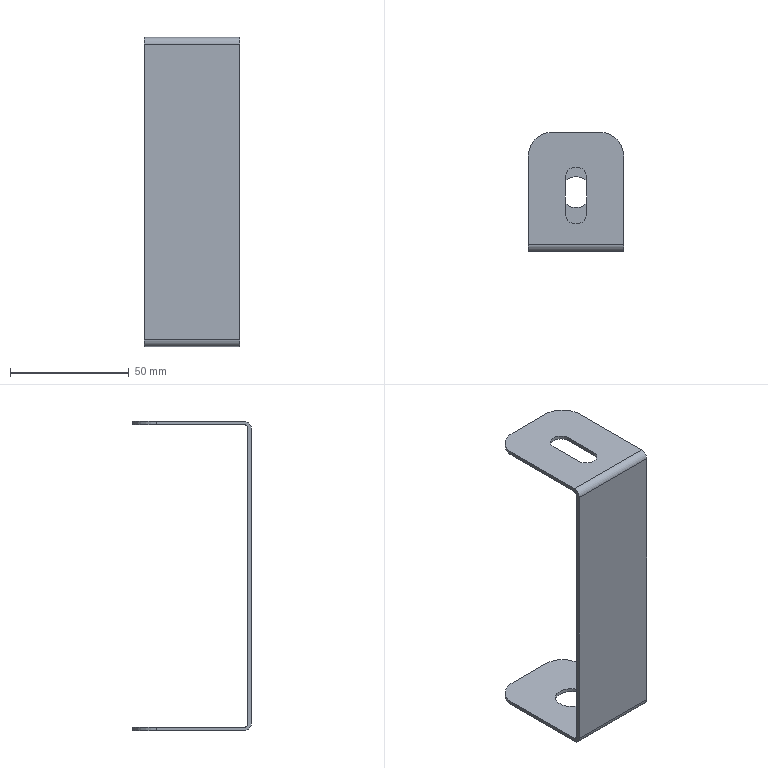Part | SolidWorks | features BaseBody 1 | 1 solid | 24 faces | box 40 x 50 x 130 mm | volume 12878 mm3 | cylinder 12 | plane 12 | commonest cylinder face diameters 20 x4 3 x2 6 x2 9 x2 13 x2
STEP:
#1=CARTESIAN_POINT('',(6.5,0.,-128.5));
#2=VERTEX_POINT('',#1);
#3=CARTESIAN_POINT('',(-6.5,0.,-128.5));
#4=VERTEX_POINT('',#3);
#5=CARTESIAN_POINT('',(0.,0.,-128.5));
#6=DIRECTION('',(0.,0.,-1.));
#7=DIRECTION('',(-1.,0.,0.));
#8=AXIS2_PLACEMENT_3D('',#5,#6,#7);
#9=CIRCLE('',#8,6.5);
#10=EDGE_CURVE('',#2,#4,#9,.T.);
#11=ORIENTED_EDGE('',*,*,#10,.F.);
#12=CARTESIAN_POINT('',(6.5,0.,-130.));
#13=VERTEX_POINT('',#12);
#14=CARTESIAN_POINT('',(6.5,0.,-120.));
#15=DIRECTION('',(0.,0.,-1.));
#16=VECTOR('',#15,1000.);
#17=LINE('',#14,#16);
#18=EDGE_CURVE('',#2,#13,#17,.T.);
#19=ORIENTED_EDGE('',*,*,#18,.T.);
#20=CARTESIAN_POINT('',(-6.5,0.,-130.));
#21=VERTEX_POINT('',#20);
#22=CARTESIAN_POINT('',(0.,0.,-130.));
#23=DIRECTION('',(0.,0.,1.));
#24=DIRECTION('',(-1.,0.,0.));
#25=AXIS2_PLACEMENT_3D('',#22,#23,#24);
#26=CIRCLE('',#25,6.5);
#27=EDGE_CURVE('',#21,#13,#26,.T.);
#28=ORIENTED_EDGE('',*,*,#27,.F.);
#29=CARTESIAN_POINT('',(-6.5,0.,-120.));
#30=DIRECTION('',(0.,0.,-1.));
#31=VECTOR('',#30,1000.);
#32=LINE('',#29,#31);
#33=EDGE_CURVE('',#4,#21,#32,.T.);
#34=ORIENTED_EDGE('',*,*,#33,.F.);
#35=EDGE_LOOP('',(#11,#19,#28,#34));
#36=FACE_OUTER_BOUND('',#35,.T.);
#37=CARTESIAN_POINT('',(0.,0.,-120.));
#38=DIRECTION('',(0.,0.,-1.));
#39=DIRECTION('',(-1.,0.,0.));
#40=AXIS2_PLACEMENT_3D('',#37,#38,#39);
#41=CYLINDRICAL_SURFACE('',#40,6.5);
#42=ADVANCED_FACE('',(#36),#41,.F.);
#43=CARTESIAN_POINT('',(20.,-25.,-127.));
#44=VERTEX_POINT('',#43);
#45=CARTESIAN_POINT('',(20.,-25.,-3.));
#46=VERTEX_POINT('',#45);
#47=CARTESIAN_POINT('',(20.,-25.,0.));
#48=DIRECTION('',(0.,0.,1.));
#49=VECTOR('',#48,1000.);
#50=LINE('',#47,#49);
#51=EDGE_CURVE('',#44,#46,#50,.T.);
#52=ORIENTED_EDGE('',*,*,#51,.T.);
#53=CARTESIAN_POINT('',(-20.,-25.,-3.));
#54=VERTEX_POINT('',#53);
#55=CARTESIAN_POINT('',(0.,-25.,-3.));
#56=DIRECTION('',(-1.,0.,0.));
#57=VECTOR('',#56,1000.);
#58=LINE('',#55,#57);
#59=EDGE_CURVE('',#46,#54,#58,.T.);
#60=ORIENTED_EDGE('',*,*,#59,.T.);
#61=CARTESIAN_POINT('',(-20.,-25.,-127.));
#62=VERTEX_POINT('',#61);
#63=CARTESIAN_POINT('',(-20.,-25.,0.));
#64=DIRECTION('',(0.,0.,-1.));
#65=VECTOR('',#64,1000.);
#66=LINE('',#63,#65);
#67=EDGE_CURVE('',#54,#62,#66,.T.);
#68=ORIENTED_EDGE('',*,*,#67,.T.);
#69=CARTESIAN_POINT('',(0.,-25.,-127.));
#70=DIRECTION('',(1.,0.,0.));
#71=VECTOR('',#70,1000.);
#72=LINE('',#69,#71);
#73=EDGE_CURVE('',#62,#44,#72,.T.);
#74=ORIENTED_EDGE('',*,*,#73,.T.);
#75=EDGE_LOOP('',(#52,#60,#68,#74));
#76=FACE_OUTER_BOUND('',#75,.T.);
#77=CARTESIAN_POINT('',(0.,-25.,0.));
#78=DIRECTION('',(0.,-1.,0.));
#79=DIRECTION('',(0.,0.,-1.));
#80=AXIS2_PLACEMENT_3D('',#77,#78,#79);
#81=PLANE('',#80);
#82=ADVANCED_FACE('',(#76),#81,.T.);
#83=ORIENTED_EDGE('',*,*,#59,.F.);
#84=CARTESIAN_POINT('',(20.,-22.,0.));
#85=VERTEX_POINT('',#84);
#86=CARTESIAN_POINT('',(20.,-22.,-3.));
#87=DIRECTION('',(-1.,0.,0.));
#88=DIRECTION('',(0.,0.,1.));
#89=AXIS2_PLACEMENT_3D('',#86,#87,#88);
#90=CIRCLE('',#89,3.);
#91=EDGE_CURVE('',#46,#85,#90,.T.);
#92=ORIENTED_EDGE('',*,*,#91,.T.);
#93=CARTESIAN_POINT('',(-20.,-22.,0.));
#94=VERTEX_POINT('',#93);
#95=CARTESIAN_POINT('',(-20.,-22.,0.));
#96=DIRECTION('',(-1.,0.,0.));
#97=VECTOR('',#96,1000.);
#98=LINE('',#95,#97);
#99=EDGE_CURVE('',#85,#94,#98,.T.);
#100=ORIENTED_EDGE('',*,*,#99,.T.);
#101=CARTESIAN_POINT('',(-20.,-22.,-3.));
#102=DIRECTION('',(1.,0.,0.));
#103=DIRECTION('',(0.,0.,1.));
#104=AXIS2_PLACEMENT_3D('',#101,#102,#103);
#105=CIRCLE('',#104,3.);
#106=EDGE_CURVE('',#94,#54,#105,.T.);
#107=ORIENTED_EDGE('',*,*,#106,.T.);
#108=EDGE_LOOP('',(#83,#92,#100,#107));
#109=FACE_OUTER_BOUND('',#108,.T.);
#110=CARTESIAN_POINT('',(-20.,-22.,-3.));
#111=DIRECTION('',(-1.,0.,0.));
#112=DIRECTION('',(0.,0.,1.));
#113=AXIS2_PLACEMENT_3D('',#110,#111,#112);
#114=CYLINDRICAL_SURFACE('',#113,3.);
#115=ADVANCED_FACE('',(#109),#114,.T.);
#116=CARTESIAN_POINT('',(20.,-23.5,-127.));
#117=VERTEX_POINT('',#116);
#118=CARTESIAN_POINT('',(20.,-23.5,-3.));
#119=VERTEX_POINT('',#118);
#120=CARTESIAN_POINT('',(20.,-23.5,-130.));
#121=DIRECTION('',(0.,0.,1.));
#122=VECTOR('',#121,1000.);
#123=LINE('',#120,#122);
#124=EDGE_CURVE('',#117,#119,#123,.T.);
#125=ORIENTED_EDGE('',*,*,#124,.T.);
#126=CARTESIAN_POINT('',(20.,-22.,-1.5));
#127=VERTEX_POINT('',#126);
#128=CARTESIAN_POINT('',(20.,-22.,-3.));
#129=DIRECTION('',(-1.,0.,0.));
#130=DIRECTION('',(0.,0.,1.));
#131=AXIS2_PLACEMENT_3D('',#128,#129,#130);
#132=CIRCLE('',#131,1.5);
#133=EDGE_CURVE('',#119,#127,#132,.T.);
#134=ORIENTED_EDGE('',*,*,#133,.T.);
#135=CARTESIAN_POINT('',(20.,15.,-1.5));
#136=VERTEX_POINT('',#135);
#137=CARTESIAN_POINT('',(20.,-25.,-1.5));
#138=DIRECTION('',(0.,1.,0.));
#139=VECTOR('',#138,1000.);
#140=LINE('',#137,#139);
#141=EDGE_CURVE('',#127,#136,#140,.T.);
#142=ORIENTED_EDGE('',*,*,#141,.T.);
#143=CARTESIAN_POINT('',(20.,15.,0.));
#144=VERTEX_POINT('',#143);
#145=CARTESIAN_POINT('',(20.,15.,-1.5));
#146=DIRECTION('',(0.,0.,1.));
#147=VECTOR('',#146,1000.);
#148=LINE('',#145,#147);
#149=EDGE_CURVE('',#136,#144,#148,.T.);
#150=ORIENTED_EDGE('',*,*,#149,.T.);
#151=CARTESIAN_POINT('',(20.,0.,0.));
#152=DIRECTION('',(0.,-1.,0.));
#153=VECTOR('',#152,1000.);
#154=LINE('',#151,#153);
#155=EDGE_CURVE('',#144,#85,#154,.T.);
#156=ORIENTED_EDGE('',*,*,#155,.T.);
#157=ORIENTED_EDGE('',*,*,#91,.F.);
#158=ORIENTED_EDGE('',*,*,#51,.F.);
#159=CARTESIAN_POINT('',(20.,-22.,-130.));
#160=VERTEX_POINT('',#159);
#161=CARTESIAN_POINT('',(20.,-22.,-127.));
#162=DIRECTION('',(-1.,0.,0.));
#163=DIRECTION('',(0.,0.,1.));
#164=AXIS2_PLACEMENT_3D('',#161,#162,#163);
#165=CIRCLE('',#164,3.);
#166=EDGE_CURVE('',#160,#44,#165,.T.);
#167=ORIENTED_EDGE('',*,*,#166,.F.);
#168=CARTESIAN_POINT('',(20.,15.,-130.));
#169=VERTEX_POINT('',#168);
#170=CARTESIAN_POINT('',(20.,0.,-130.));
#171=DIRECTION('',(0.,-1.,0.));
#172=VECTOR('',#171,1000.);
#173=LINE('',#170,#172);
#174=EDGE_CURVE('',#169,#160,#173,.T.);
#175=ORIENTED_EDGE('',*,*,#174,.F.);
#176=CARTESIAN_POINT('',(20.,15.,-128.5));
#177=VERTEX_POINT('',#176);
#178=CARTESIAN_POINT('',(20.,15.,-130.));
#179=DIRECTION('',(0.,0.,1.));
#180=VECTOR('',#179,1000.);
#181=LINE('',#178,#180);
#182=EDGE_CURVE('',#169,#177,#181,.T.);
#183=ORIENTED_EDGE('',*,*,#182,.T.);
#184=CARTESIAN_POINT('',(20.,-22.,-128.5));
#185=VERTEX_POINT('',#184);
#186=CARTESIAN_POINT('',(20.,25.,-128.5));
#187=DIRECTION('',(0.,-1.,0.));
#188=VECTOR('',#187,1000.);
#189=LINE('',#186,#188);
#190=EDGE_CURVE('',#177,#185,#189,.T.);
#191=ORIENTED_EDGE('',*,*,#190,.T.);
#192=CARTESIAN_POINT('',(20.,-22.,-127.));
#193=DIRECTION('',(-1.,0.,0.));
#194=DIRECTION('',(0.,0.,1.));
#195=AXIS2_PLACEMENT_3D('',#192,#193,#194);
#196=CIRCLE('',#195,1.5);
#197=EDGE_CURVE('',#185,#117,#196,.T.);
#198=ORIENTED_EDGE('',*,*,#197,.T.);
#199=EDGE_LOOP('',(#125,#134,#142,#150,#156,#157,#158,#167,#175,#183,#191,#198));
#200=FACE_OUTER_BOUND('',#199,.T.);
#201=CARTESIAN_POINT('',(20.,-25.,-130.));
#202=DIRECTION('',(1.,0.,0.));
#203=DIRECTION('',(0.,0.,-1.));
#204=AXIS2_PLACEMENT_3D('',#201,#202,#203);
#205=PLANE('',#204);
#206=ADVANCED_FACE('',(#200),#205,.T.);
#207=CARTESIAN_POINT('',(-20.,-22.,-130.));
#208=VERTEX_POINT('',#207);
#209=CARTESIAN_POINT('',(-20.,-22.,-130.));
#210=DIRECTION('',(1.,0.,0.));
#211=VECTOR('',#210,1000.);
#212=LINE('',#209,#211);
#213=EDGE_CURVE('',#208,#160,#212,.T.);
#214=ORIENTED_EDGE('',*,*,#213,.T.);
#215=ORIENTED_EDGE('',*,*,#166,.T.);
#216=ORIENTED_EDGE('',*,*,#73,.F.);
#217=CARTESIAN_POINT('',(-20.,-22.,-127.));
#218=DIRECTION('',(1.,0.,0.));
#219=DIRECTION('',(0.,0.,1.));
#220=AXIS2_PLACEMENT_3D('',#217,#218,#219);
#221=CIRCLE('',#220,3.);
#222=EDGE_CURVE('',#62,#208,#221,.T.);
#223=ORIENTED_EDGE('',*,*,#222,.T.);
#224=EDGE_LOOP('',(#214,#215,#216,#223));
#225=FACE_OUTER_BOUND('',#224,.T.);
#226=CARTESIAN_POINT('',(-20.,-22.,-127.));
#227=DIRECTION('',(-1.,0.,0.));
#228=DIRECTION('',(0.,0.,1.));
#229=AXIS2_PLACEMENT_3D('',#226,#227,#228);
#230=CYLINDRICAL_SURFACE('',#229,3.);
#231=ADVANCED_FACE('',(#225),#230,.T.);
#232=ORIENTED_EDGE('',*,*,#67,.F.);
#233=ORIENTED_EDGE('',*,*,#106,.F.);
#234=CARTESIAN_POINT('',(-20.,15.,0.));
#235=VERTEX_POINT('',#234);
#236=CARTESIAN_POINT('',(-20.,0.,0.));
#237=DIRECTION('',(0.,1.,0.));
#238=VECTOR('',#237,1000.);
#239=LINE('',#236,#238);
#240=EDGE_CURVE('',#94,#235,#239,.T.);
#241=ORIENTED_EDGE('',*,*,#240,.T.);
#242=CARTESIAN_POINT('',(-20.,15.,-1.5));
#243=VERTEX_POINT('',#242);
#244=CARTESIAN_POINT('',(-20.,15.,-1.5));
#245=DIRECTION('',(0.,0.,1.));
#246=VECTOR('',#245,1000.);
#247=LINE('',#244,#246);
#248=EDGE_CURVE('',#243,#235,#247,.T.);
#249=ORIENTED_EDGE('',*,*,#248,.F.);
#250=CARTESIAN_POINT('',(-20.,-22.,-1.5));
#251=VERTEX_POINT('',#250);
#252=CARTESIAN_POINT('',(-20.,-25.,-1.5));
#253=DIRECTION('',(0.,-1.,0.));
#254=VECTOR('',#253,1000.);
#255=LINE('',#252,#254);
#256=EDGE_CURVE('',#243,#251,#255,.T.);
#257=ORIENTED_EDGE('',*,*,#256,.T.);
#258=CARTESIAN_POINT('',(-20.,-23.5,-3.));
#259=VERTEX_POINT('',#258);
#260=CARTESIAN_POINT('',(-20.,-22.,-3.));
#261=DIRECTION('',(-1.,0.,0.));
#262=DIRECTION('',(0.,0.,1.));
#263=AXIS2_PLACEMENT_3D('',#260,#261,#262);
#264=CIRCLE('',#263,1.5);
#265=EDGE_CURVE('',#259,#251,#264,.T.);
#266=ORIENTED_EDGE('',*,*,#265,.F.);
#267=CARTESIAN_POINT('',(-20.,-23.5,-127.));
#268=VERTEX_POINT('',#267);
#269=CARTESIAN_POINT('',(-20.,-23.5,-1.5));
#270=DIRECTION('',(0.,0.,-1.));
#271=VECTOR('',#270,1000.);
#272=LINE('',#269,#271);
#273=EDGE_CURVE('',#259,#268,#272,.T.);
#274=ORIENTED_EDGE('',*,*,#273,.T.);
#275=CARTESIAN_POINT('',(-20.,-22.,-128.5));
#276=VERTEX_POINT('',#275);
#277=CARTESIAN_POINT('',(-20.,-22.,-127.));
#278=DIRECTION('',(-1.,0.,0.));
#279=DIRECTION('',(0.,0.,1.));
#280=AXIS2_PLACEMENT_3D('',#277,#278,#279);
#281=CIRCLE('',#280,1.5);
#282=EDGE_CURVE('',#276,#268,#281,.T.);
#283=ORIENTED_EDGE('',*,*,#282,.F.);
#284=CARTESIAN_POINT('',(-20.,15.,-128.5));
#285=VERTEX_POINT('',#284);
#286=CARTESIAN_POINT('',(-20.,-23.5,-128.5));
#287=DIRECTION('',(0.,1.,0.));
#288=VECTOR('',#287,1000.);
#289=LINE('',#286,#288);
#290=EDGE_CURVE('',#276,#285,#289,.T.);
#291=ORIENTED_EDGE('',*,*,#290,.T.);
#292=CARTESIAN_POINT('',(-20.,15.,-130.));
#293=VERTEX_POINT('',#292);
#294=CARTESIAN_POINT('',(-20.,15.,-130.));
#295=DIRECTION('',(0.,0.,1.));
#296=VECTOR('',#295,1000.);
#297=LINE('',#294,#296);
#298=EDGE_CURVE('',#293,#285,#297,.T.);
#299=ORIENTED_EDGE('',*,*,#298,.F.);
#300=CARTESIAN_POINT('',(-20.,0.,-130.));
#301=DIRECTION('',(0.,1.,0.));
#302=VECTOR('',#301,1000.);
#303=LINE('',#300,#302);
#304=EDGE_CURVE('',#208,#293,#303,.T.);
#305=ORIENTED_EDGE('',*,*,#304,.F.);
#306=ORIENTED_EDGE('',*,*,#222,.F.);
#307=EDGE_LOOP('',(#232,#233,#241,#249,#257,#266,#274,#283,#291,#299,#305,#306));
#308=FACE_OUTER_BOUND('',#307,.T.);
#309=CARTESIAN_POINT('',(-20.,-25.,-1.5));
#310=DIRECTION('',(-1.,0.,0.));
#311=DIRECTION('',(0.,0.,1.));
#312=AXIS2_PLACEMENT_3D('',#309,#310,#311);
#313=PLANE('',#312);
#314=ADVANCED_FACE('',(#308),#313,.T.);
#315=CARTESIAN_POINT('',(-10.,25.,0.));
#316=VERTEX_POINT('',#315);
#317=CARTESIAN_POINT('',(-10.,15.,0.));
#318=DIRECTION('',(0.,0.,-1.));
#319=DIRECTION('',(1.,0.,0.));
#320=AXIS2_PLACEMENT_3D('',#317,#318,#319);
#321=CIRCLE('',#320,10.);
#322=EDGE_CURVE('',#235,#316,#321,.T.);
#323=ORIENTED_EDGE('',*,*,#322,.F.);
#324=ORIENTED_EDGE('',*,*,#240,.F.);
#325=ORIENTED_EDGE('',*,*,#99,.F.);
#326=ORIENTED_EDGE('',*,*,#155,.F.);
#327=CARTESIAN_POINT('',(10.,25.,0.));
#328=VERTEX_POINT('',#327);
#329=CARTESIAN_POINT('',(10.,15.,0.));
#330=DIRECTION('',(0.,0.,-1.));
#331=DIRECTION('',(1.,0.,0.));
#332=AXIS2_PLACEMENT_3D('',#329,#330,#331);
#333=CIRCLE('',#332,10.);
#334=EDGE_CURVE('',#328,#144,#333,.T.);
#335=ORIENTED_EDGE('',*,*,#334,.F.);
#336=CARTESIAN_POINT('',(0.,25.,0.));
#337=DIRECTION('',(1.,0.,0.));
#338=VECTOR('',#337,1000.);
#339=LINE('',#336,#338);
#340=EDGE_CURVE('',#316,#328,#339,.T.);
#341=ORIENTED_EDGE('',*,*,#340,.F.);
#342=EDGE_LOOP('',(#323,#324,#325,#326,#335,#341));
#343=FACE_OUTER_BOUND('',#342,.T.);
#344=CARTESIAN_POINT('',(4.5,5.927,0.));
#345=VERTEX_POINT('',#344);
#346=CARTESIAN_POINT('',(-4.5,5.927,0.));
#347=VERTEX_POINT('',#346);
#348=CARTESIAN_POINT('',(0.,5.927,0.));
#349=DIRECTION('',(0.,0.,1.));
#350=DIRECTION('',(1.,0.,0.));
#351=AXIS2_PLACEMENT_3D('',#348,#349,#350);
#352=CIRCLE('',#351,4.5);
#353=EDGE_CURVE('',#345,#347,#352,.T.);
#354=ORIENTED_EDGE('',*,*,#353,.F.);
#355=CARTESIAN_POINT('',(4.5,-9.073,0.));
#356=VERTEX_POINT('',#355);
#357=CARTESIAN_POINT('',(4.5,0.,0.));
#358=DIRECTION('',(0.,1.,0.));
#359=VECTOR('',#358,1000.);
#360=LINE('',#357,#359);
#361=EDGE_CURVE('',#356,#345,#360,.T.);
#362=ORIENTED_EDGE('',*,*,#361,.F.);
#363=CARTESIAN_POINT('',(-4.5,-9.073,0.));
#364=VERTEX_POINT('',#363);
#365=CARTESIAN_POINT('',(0.,-9.073,0.));
#366=DIRECTION('',(0.,0.,1.));
#367=DIRECTION('',(1.,0.,0.));
#368=AXIS2_PLACEMENT_3D('',#365,#366,#367);
#369=CIRCLE('',#368,4.5);
#370=EDGE_CURVE('',#364,#356,#369,.T.);
#371=ORIENTED_EDGE('',*,*,#370,.F.);
#372=CARTESIAN_POINT('',(-4.5,0.,0.));
#373=DIRECTION('',(0.,-1.,0.));
#374=VECTOR('',#373,1000.);
#375=LINE('',#372,#374);
#376=EDGE_CURVE('',#347,#364,#375,.T.);
#377=ORIENTED_EDGE('',*,*,#376,.F.);
#378=EDGE_LOOP('',(#354,#362,#371,#377));
#379=FACE_BOUND('',#378,.T.);
#380=CARTESIAN_POINT('',(0.,0.,0.));
#381=DIRECTION('',(0.,0.,-1.));
#382=DIRECTION('',(-1.,0.,0.));
#383=AXIS2_PLACEMENT_3D('',#380,#381,#382);
#384=PLANE('',#383);
#385=ADVANCED_FACE('',(#343,#379),#384,.F.);
#386=ORIENTED_EDGE('',*,*,#273,.F.);
#387=CARTESIAN_POINT('',(0.,-23.5,-3.));
#388=DIRECTION('',(-1.,0.,0.));
#389=VECTOR('',#388,1000.);
#390=LINE('',#387,#389);
#391=EDGE_CURVE('',#119,#259,#390,.T.);
#392=ORIENTED_EDGE('',*,*,#391,.F.);
#393=ORIENTED_EDGE('',*,*,#124,.F.);
#394=CARTESIAN_POINT('',(0.,-23.5,-127.));
#395=DIRECTION('',(1.,0.,0.));
#396=VECTOR('',#395,1000.);
#397=LINE('',#394,#396);
#398=EDGE_CURVE('',#268,#117,#397,.T.);
#399=ORIENTED_EDGE('',*,*,#398,.F.);
#400=EDGE_LOOP('',(#386,#392,#393,#399));
#401=FACE_OUTER_BOUND('',#400,.T.);
#402=CARTESIAN_POINT('',(0.,-23.5,0.));
#403=DIRECTION('',(0.,-1.,0.));
#404=DIRECTION('',(0.,0.,-1.));
#405=AXIS2_PLACEMENT_3D('',#402,#403,#404);
#406=PLANE('',#405);
#407=ADVANCED_FACE('',(#401),#406,.F.);
#408=ORIENTED_EDGE('',*,*,#304,.T.);
#409=CARTESIAN_POINT('',(-10.,25.,-130.));
#410=VERTEX_POINT('',#409);
#411=CARTESIAN_POINT('',(-10.,15.,-130.));
#412=DIRECTION('',(0.,0.,-1.));
#413=DIRECTION('',(1.,0.,0.));
#414=AXIS2_PLACEMENT_3D('',#411,#412,#413);
#415=CIRCLE('',#414,10.);
#416=EDGE_CURVE('',#293,#410,#415,.T.);
#417=ORIENTED_EDGE('',*,*,#416,.T.);
#418=CARTESIAN_POINT('',(10.,25.,-130.));
#419=VERTEX_POINT('',#418);
#420=CARTESIAN_POINT('',(0.,25.,-130.));
#421=DIRECTION('',(1.,0.,0.));
#422=VECTOR('',#421,1000.);
#423=LINE('',#420,#422);
#424=EDGE_CURVE('',#410,#419,#423,.T.);
#425=ORIENTED_EDGE('',*,*,#424,.T.);
#426=CARTESIAN_POINT('',(10.,15.,-130.));
#427=DIRECTION('',(0.,0.,-1.));
#428=DIRECTION('',(1.,0.,0.));
#429=AXIS2_PLACEMENT_3D('',#426,#427,#428);
#430=CIRCLE('',#429,10.);
#431=EDGE_CURVE('',#419,#169,#430,.T.);
#432=ORIENTED_EDGE('',*,*,#431,.T.);
#433=ORIENTED_EDGE('',*,*,#174,.T.);
#434=ORIENTED_EDGE('',*,*,#213,.F.);
#435=EDGE_LOOP('',(#408,#417,#425,#432,#433,#434));
#436=FACE_OUTER_BOUND('',#435,.T.);
#437=ORIENTED_EDGE('',*,*,#27,.T.);
#438=CARTESIAN_POINT('',(0.,0.,-130.));
#439=DIRECTION('',(0.,0.,1.));
#440=DIRECTION('',(-1.,0.,0.));
#441=AXIS2_PLACEMENT_3D('',#438,#439,#440);
#442=CIRCLE('',#441,6.5);
#443=EDGE_CURVE('',#13,#21,#442,.T.);
#444=ORIENTED_EDGE('',*,*,#443,.T.);
#445=EDGE_LOOP('',(#437,#444));
#446=FACE_BOUND('',#445,.T.);
#447=CARTESIAN_POINT('',(0.,0.,-130.));
#448=DIRECTION('',(0.,0.,-1.));
#449=DIRECTION('',(-1.,0.,0.));
#450=AXIS2_PLACEMENT_3D('',#447,#448,#449);
#451=PLANE('',#450);
#452=ADVANCED_FACE('',(#436,#446),#451,.T.);
#453=ORIENTED_EDGE('',*,*,#133,.F.);
#454=ORIENTED_EDGE('',*,*,#391,.T.);
#455=ORIENTED_EDGE('',*,*,#265,.T.);
#456=CARTESIAN_POINT('',(-20.,-22.,-1.5));
#457=DIRECTION('',(-1.,0.,0.));
#458=VECTOR('',#457,1000.);
#459=LINE('',#456,#458);
#460=EDGE_CURVE('',#127,#251,#459,.T.);
#461=ORIENTED_EDGE('',*,*,#460,.F.);
#462=EDGE_LOOP('',(#453,#454,#455,#461));
#463=FACE_OUTER_BOUND('',#462,.T.);
#464=CARTESIAN_POINT('',(-20.,-22.,-3.));
#465=DIRECTION('',(-1.,0.,0.));
#466=DIRECTION('',(0.,0.,1.));
#467=AXIS2_PLACEMENT_3D('',#464,#465,#466);
#468=CYLINDRICAL_SURFACE('',#467,1.5);
#469=ADVANCED_FACE('',(#463),#468,.F.);
#470=ORIENTED_EDGE('',*,*,#340,.T.);
#471=CARTESIAN_POINT('',(10.,25.,-1.5));
#472=VERTEX_POINT('',#471);
#473=CARTESIAN_POINT('',(10.,25.,-1.5));
#474=DIRECTION('',(0.,0.,-1.));
#475=VECTOR('',#474,1000.);
#476=LINE('',#473,#475);
#477=EDGE_CURVE('',#328,#472,#476,.T.);
#478=ORIENTED_EDGE('',*,*,#477,.T.);
#479=CARTESIAN_POINT('',(-10.,25.,-1.5));
#480=VERTEX_POINT('',#479);
#481=CARTESIAN_POINT('',(-20.,25.,-1.5));
#482=DIRECTION('',(-1.,0.,0.));
#483=VECTOR('',#482,1000.);
#484=LINE('',#481,#483);
#485=EDGE_CURVE('',#472,#480,#484,.T.);
#486=ORIENTED_EDGE('',*,*,#485,.T.);
#487=CARTESIAN_POINT('',(-10.,25.,-1.5));
#488=DIRECTION('',(0.,0.,1.));
#489=VECTOR('',#488,1000.);
#490=LINE('',#487,#489);
#491=EDGE_CURVE('',#480,#316,#490,.T.);
#492=ORIENTED_EDGE('',*,*,#491,.T.);
#493=EDGE_LOOP('',(#470,#478,#486,#492));
#494=FACE_OUTER_BOUND('',#493,.T.);
#495=CARTESIAN_POINT('',(-20.,25.,-1.5));
#496=DIRECTION('',(0.,1.,0.));
#497=DIRECTION('',(0.,0.,1.));
#498=AXIS2_PLACEMENT_3D('',#495,#496,#497);
#499=PLANE('',#498);
#500=ADVANCED_FACE('',(#494),#499,.T.);
#501=ORIENTED_EDGE('',*,*,#322,.T.);
#502=ORIENTED_EDGE('',*,*,#491,.F.);
#503=CARTESIAN_POINT('',(-10.,15.,-1.5));
#504=DIRECTION('',(0.,0.,1.));
#505=DIRECTION('',(1.,0.,0.));
#506=AXIS2_PLACEMENT_3D('',#503,#504,#505);
#507=CIRCLE('',#506,10.);
#508=EDGE_CURVE('',#480,#243,#507,.T.);
#509=ORIENTED_EDGE('',*,*,#508,.T.);
#510=ORIENTED_EDGE('',*,*,#248,.T.);
#511=EDGE_LOOP('',(#501,#502,#509,#510));
#512=FACE_OUTER_BOUND('',#511,.T.);
#513=CARTESIAN_POINT('',(-10.,15.,-1.5));
#514=DIRECTION('',(0.,0.,1.));
#515=DIRECTION('',(1.,0.,0.));
#516=AXIS2_PLACEMENT_3D('',#513,#514,#515);
#517=CYLINDRICAL_SURFACE('',#516,10.);
#518=ADVANCED_FACE('',(#512),#517,.T.);
#519=ORIENTED_EDGE('',*,*,#334,.T.);
#520=ORIENTED_EDGE('',*,*,#149,.F.);
#521=CARTESIAN_POINT('',(10.,15.,-1.5));
#522=DIRECTION('',(0.,0.,1.));
#523=DIRECTION('',(1.,0.,0.));
#524=AXIS2_PLACEMENT_3D('',#521,#522,#523);
#525=CIRCLE('',#524,10.);
#526=EDGE_CURVE('',#136,#472,#525,.T.);
#527=ORIENTED_EDGE('',*,*,#526,.T.);
#528=ORIENTED_EDGE('',*,*,#477,.F.);
#529=EDGE_LOOP('',(#519,#520,#527,#528));
#530=FACE_OUTER_BOUND('',#529,.T.);
#531=CARTESIAN_POINT('',(10.,15.,-1.5));
#532=DIRECTION('',(0.,0.,1.));
#533=DIRECTION('',(1.,0.,0.));
#534=AXIS2_PLACEMENT_3D('',#531,#532,#533);
#535=CYLINDRICAL_SURFACE('',#534,10.);
#536=ADVANCED_FACE('',(#530),#535,.T.);
#537=CARTESIAN_POINT('',(-4.5,5.927,-1.5));
#538=VERTEX_POINT('',#537);
#539=CARTESIAN_POINT('',(-4.5,5.927,-10.));
#540=DIRECTION('',(0.,0.,-1.));
#541=VECTOR('',#540,1000.);
#542=LINE('',#539,#541);
#543=EDGE_CURVE('',#347,#538,#542,.T.);
#544=ORIENTED_EDGE('',*,*,#543,.F.);
#545=ORIENTED_EDGE('',*,*,#376,.T.);
#546=CARTESIAN_POINT('',(-4.5,-9.073,-1.5));
#547=VERTEX_POINT('',#546);
#548=CARTESIAN_POINT('',(-4.5,-9.073,-10.));
#549=DIRECTION('',(0.,0.,1.));
#550=VECTOR('',#549,1000.);
#551=LINE('',#548,#550);
#552=EDGE_CURVE('',#547,#364,#551,.T.);
#553=ORIENTED_EDGE('',*,*,#552,.F.);
#554=CARTESIAN_POINT('',(-4.5,5.927,-1.5));
#555=DIRECTION('',(0.,-1.,0.));
#556=VECTOR('',#555,1000.);
#557=LINE('',#554,#556);
#558=EDGE_CURVE('',#538,#547,#557,.T.);
#559=ORIENTED_EDGE('',*,*,#558,.F.);
#560=EDGE_LOOP('',(#544,#545,#553,#559));
#561=FACE_OUTER_BOUND('',#560,.T.);
#562=CARTESIAN_POINT('',(-4.5,5.927,-10.));
#563=DIRECTION('',(-1.,0.,0.));
#564=DIRECTION('',(0.,-1.,0.));
#565=AXIS2_PLACEMENT_3D('',#562,#563,#564);
#566=PLANE('',#565);
#567=ADVANCED_FACE('',(#561),#566,.F.);
#568=CARTESIAN_POINT('',(4.5,5.927,-1.5));
#569=VERTEX_POINT('',#568);
#570=CARTESIAN_POINT('',(4.5,5.927,-10.));
#571=DIRECTION('',(0.,0.,-1.));
#572=VECTOR('',#571,1000.);
#573=LINE('',#570,#572);
#574=EDGE_CURVE('',#345,#569,#573,.T.);
#575=ORIENTED_EDGE('',*,*,#574,.F.);
#576=ORIENTED_EDGE('',*,*,#353,.T.);
#577=ORIENTED_EDGE('',*,*,#543,.T.);
#578=CARTESIAN_POINT('',(0.,5.927,-1.5));
#579=DIRECTION('',(0.,0.,1.));
#580=DIRECTION('',(1.,0.,0.));
#581=AXIS2_PLACEMENT_3D('',#578,#579,#580);
#582=CIRCLE('',#581,4.5);
#583=EDGE_CURVE('',#569,#538,#582,.T.);
#584=ORIENTED_EDGE('',*,*,#583,.F.);
#585=EDGE_LOOP('',(#575,#576,#577,#584));
#586=FACE_OUTER_BOUND('',#585,.T.);
#587=CARTESIAN_POINT('',(0.,5.927,-10.));
#588=DIRECTION('',(0.,0.,1.));
#589=DIRECTION('',(1.,0.,0.));
#590=AXIS2_PLACEMENT_3D('',#587,#588,#589);
#591=CYLINDRICAL_SURFACE('',#590,4.5);
#592=ADVANCED_FACE('',(#586),#591,.F.);
#593=CARTESIAN_POINT('',(4.5,-9.073,-1.5));
#594=VERTEX_POINT('',#593);
#595=CARTESIAN_POINT('',(4.5,-9.073,-10.));
#596=DIRECTION('',(0.,0.,-1.));
#597=VECTOR('',#596,1000.);
#598=LINE('',#595,#597);
#599=EDGE_CURVE('',#356,#594,#598,.T.);
#600=ORIENTED_EDGE('',*,*,#599,.F.);
#601=ORIENTED_EDGE('',*,*,#361,.T.);
#602=ORIENTED_EDGE('',*,*,#574,.T.);
#603=CARTESIAN_POINT('',(4.5,5.927,-1.5));
#604=DIRECTION('',(0.,1.,0.));
#605=VECTOR('',#604,1000.);
#606=LINE('',#603,#605);
#607=EDGE_CURVE('',#594,#569,#606,.T.);
#608=ORIENTED_EDGE('',*,*,#607,.F.);
#609=EDGE_LOOP('',(#600,#601,#602,#608));
#610=FACE_OUTER_BOUND('',#609,.T.);
#611=CARTESIAN_POINT('',(4.5,5.927,-10.));
#612=DIRECTION('',(1.,0.,0.));
#613=DIRECTION('',(0.,1.,0.));
#614=AXIS2_PLACEMENT_3D('',#611,#612,#613);
#615=PLANE('',#614);
#616=ADVANCED_FACE('',(#610),#615,.F.);
#617=ORIENTED_EDGE('',*,*,#552,.T.);
#618=ORIENTED_EDGE('',*,*,#370,.T.);
#619=ORIENTED_EDGE('',*,*,#599,.T.);
#620=CARTESIAN_POINT('',(0.,-9.073,-1.5));
#621=DIRECTION('',(0.,0.,1.));
#622=DIRECTION('',(1.,0.,0.));
#623=AXIS2_PLACEMENT_3D('',#620,#621,#622);
#624=CIRCLE('',#623,4.5);
#625=EDGE_CURVE('',#547,#594,#624,.T.);
#626=ORIENTED_EDGE('',*,*,#625,.F.);
#627=EDGE_LOOP('',(#617,#618,#619,#626));
#628=FACE_OUTER_BOUND('',#627,.T.);
#629=CARTESIAN_POINT('',(0.,-9.073,-10.));
#630=DIRECTION('',(0.,0.,1.));
#631=DIRECTION('',(1.,0.,0.));
#632=AXIS2_PLACEMENT_3D('',#629,#630,#631);
#633=CYLINDRICAL_SURFACE('',#632,4.5);
#634=ADVANCED_FACE('',(#628),#633,.F.);
#635=ORIENTED_EDGE('',*,*,#197,.F.);
#636=CARTESIAN_POINT('',(-20.,-22.,-128.5));
#637=DIRECTION('',(1.,0.,0.));
#638=VECTOR('',#637,1000.);
#639=LINE('',#636,#638);
#640=EDGE_CURVE('',#276,#185,#639,.T.);
#641=ORIENTED_EDGE('',*,*,#640,.F.);
#642=ORIENTED_EDGE('',*,*,#282,.T.);
#643=ORIENTED_EDGE('',*,*,#398,.T.);
#644=EDGE_LOOP('',(#635,#641,#642,#643));
#645=FACE_OUTER_BOUND('',#644,.T.);
#646=CARTESIAN_POINT('',(-20.,-22.,-127.));
#647=DIRECTION('',(-1.,0.,0.));
#648=DIRECTION('',(0.,0.,1.));
#649=AXIS2_PLACEMENT_3D('',#646,#647,#648);
#650=CYLINDRICAL_SURFACE('',#649,1.5);
#651=ADVANCED_FACE('',(#645),#650,.F.);
#652=CARTESIAN_POINT('',(-10.,25.,-128.5));
#653=VERTEX_POINT('',#652);
#654=CARTESIAN_POINT('',(-10.,15.,-128.5));
#655=DIRECTION('',(0.,0.,-1.));
#656=DIRECTION('',(1.,0.,0.));
#657=AXIS2_PLACEMENT_3D('',#654,#655,#656);
#658=CIRCLE('',#657,10.);
#659=EDGE_CURVE('',#285,#653,#658,.T.);
#660=ORIENTED_EDGE('',*,*,#659,.T.);
#661=CARTESIAN_POINT('',(-10.,25.,-130.));
#662=DIRECTION('',(0.,0.,-1.));
#663=VECTOR('',#662,1000.);
#664=LINE('',#661,#663);
#665=EDGE_CURVE('',#653,#410,#664,.T.);
#666=ORIENTED_EDGE('',*,*,#665,.T.);
#667=ORIENTED_EDGE('',*,*,#416,.F.);
#668=ORIENTED_EDGE('',*,*,#298,.T.);
#669=EDGE_LOOP('',(#660,#666,#667,#668));
#670=FACE_OUTER_BOUND('',#669,.T.);
#671=CARTESIAN_POINT('',(-10.,15.,-130.));
#672=DIRECTION('',(0.,0.,1.));
#673=DIRECTION('',(1.,0.,0.));
#674=AXIS2_PLACEMENT_3D('',#671,#672,#673);
#675=CYLINDRICAL_SURFACE('',#674,10.);
#676=ADVANCED_FACE('',(#670),#675,.T.);
#677=CARTESIAN_POINT('',(10.,25.,-128.5));
#678=VERTEX_POINT('',#677);
#679=CARTESIAN_POINT('',(10.,15.,-128.5));
#680=DIRECTION('',(0.,0.,-1.));
#681=DIRECTION('',(1.,0.,0.));
#682=AXIS2_PLACEMENT_3D('',#679,#680,#681);
#683=CIRCLE('',#682,10.);
#684=EDGE_CURVE('',#678,#177,#683,.T.);
#685=ORIENTED_EDGE('',*,*,#684,.T.);
#686=ORIENTED_EDGE('',*,*,#182,.F.);
#687=ORIENTED_EDGE('',*,*,#431,.F.);
#688=CARTESIAN_POINT('',(10.,25.,-130.));
#689=DIRECTION('',(0.,0.,1.));
#690=VECTOR('',#689,1000.);
#691=LINE('',#688,#690);
#692=EDGE_CURVE('',#419,#678,#691,.T.);
#693=ORIENTED_EDGE('',*,*,#692,.T.);
#694=EDGE_LOOP('',(#685,#686,#687,#693));
#695=FACE_OUTER_BOUND('',#694,.T.);
#696=CARTESIAN_POINT('',(10.,15.,-130.));
#697=DIRECTION('',(0.,0.,1.));
#698=DIRECTION('',(1.,0.,0.));
#699=AXIS2_PLACEMENT_3D('',#696,#697,#698);
#700=CYLINDRICAL_SURFACE('',#699,10.);
#701=ADVANCED_FACE('',(#695),#700,.T.);
#702=ORIENTED_EDGE('',*,*,#424,.F.);
#703=ORIENTED_EDGE('',*,*,#665,.F.);
#704=CARTESIAN_POINT('',(-20.,25.,-128.5));
#705=DIRECTION('',(1.,0.,0.));
#706=VECTOR('',#705,1000.);
#707=LINE('',#704,#706);
#708=EDGE_CURVE('',#653,#678,#707,.T.);
#709=ORIENTED_EDGE('',*,*,#708,.T.);
#710=ORIENTED_EDGE('',*,*,#692,.F.);
#711=EDGE_LOOP('',(#702,#703,#709,#710));
#712=FACE_OUTER_BOUND('',#711,.T.);
#713=CARTESIAN_POINT('',(-20.,25.,-130.));
#714=DIRECTION('',(0.,1.,0.));
#715=DIRECTION('',(0.,0.,1.));
#716=AXIS2_PLACEMENT_3D('',#713,#714,#715);
#717=PLANE('',#716);
#718=ADVANCED_FACE('',(#712),#717,.T.);
#719=ORIENTED_EDGE('',*,*,#18,.F.);
#720=CARTESIAN_POINT('',(0.,0.,-128.5));
#721=DIRECTION('',(0.,0.,-1.));
#722=DIRECTION('',(-1.,0.,0.));
#723=AXIS2_PLACEMENT_3D('',#720,#721,#722);
#724=CIRCLE('',#723,6.5);
#725=EDGE_CURVE('',#4,#2,#724,.T.);
#726=ORIENTED_EDGE('',*,*,#725,.F.);
#727=ORIENTED_EDGE('',*,*,#33,.T.);
#728=ORIENTED_EDGE('',*,*,#443,.F.);
#729=EDGE_LOOP('',(#719,#726,#727,#728));
#730=FACE_OUTER_BOUND('',#729,.T.);
#731=CARTESIAN_POINT('',(0.,0.,-120.));
#732=DIRECTION('',(0.,0.,-1.));
#733=DIRECTION('',(-1.,0.,0.));
#734=AXIS2_PLACEMENT_3D('',#731,#732,#733);
#735=CYLINDRICAL_SURFACE('',#734,6.5);
#736=ADVANCED_FACE('',(#730),#735,.F.);
#737=ORIENTED_EDGE('',*,*,#141,.F.);
#738=ORIENTED_EDGE('',*,*,#460,.T.);
#739=ORIENTED_EDGE('',*,*,#256,.F.);
#740=ORIENTED_EDGE('',*,*,#508,.F.);
#741=ORIENTED_EDGE('',*,*,#485,.F.);
#742=ORIENTED_EDGE('',*,*,#526,.F.);
#743=EDGE_LOOP('',(#737,#738,#739,#740,#741,#742));
#744=FACE_OUTER_BOUND('',#743,.T.);
#745=ORIENTED_EDGE('',*,*,#625,.T.);
#746=ORIENTED_EDGE('',*,*,#607,.T.);
#747=ORIENTED_EDGE('',*,*,#583,.T.);
#748=ORIENTED_EDGE('',*,*,#558,.T.);
#749=EDGE_LOOP('',(#745,#746,#747,#748));
#750=FACE_BOUND('',#749,.T.);
#751=CARTESIAN_POINT('',(0.,0.,-1.5));
#752=DIRECTION('',(0.,0.,-1.));
#753=DIRECTION('',(-1.,0.,0.));
#754=AXIS2_PLACEMENT_3D('',#751,#752,#753);
#755=PLANE('',#754);
#756=ADVANCED_FACE('',(#744,#750),#755,.T.);
#757=ORIENTED_EDGE('',*,*,#684,.F.);
#758=ORIENTED_EDGE('',*,*,#708,.F.);
#759=ORIENTED_EDGE('',*,*,#659,.F.);
#760=ORIENTED_EDGE('',*,*,#290,.F.);
#761=ORIENTED_EDGE('',*,*,#640,.T.);
#762=ORIENTED_EDGE('',*,*,#190,.F.);
#763=EDGE_LOOP('',(#757,#758,#759,#760,#761,#762));
#764=FACE_OUTER_BOUND('',#763,.T.);
#765=ORIENTED_EDGE('',*,*,#725,.T.);
#766=ORIENTED_EDGE('',*,*,#10,.T.);
#767=EDGE_LOOP('',(#765,#766));
#768=FACE_BOUND('',#767,.T.);
#769=CARTESIAN_POINT('',(0.,0.,-128.5));
#770=DIRECTION('',(0.,0.,-1.));
#771=DIRECTION('',(-1.,0.,0.));
#772=AXIS2_PLACEMENT_3D('',#769,#770,#771);
#773=PLANE('',#772);
#774=ADVANCED_FACE('',(#764,#768),#773,.F.);
#775=CLOSED_SHELL('',(#42,#82,#115,#206,#231,#314,#385,#407,#452,#469,#500,#518,#536,#567,#592,#616,#634,#651,#676,#701,#718,#736,#756,#774));
#776=MANIFOLD_SOLID_BREP('',#775);
#777=CARTESIAN_POINT('',(0.,0.,0.));
#778=DIRECTION('',(0.,0.,1.));
#779=DIRECTION('',(1.,0.,0.));
#780=AXIS2_PLACEMENT_3D('',#777,#778,#779);
#781=(LENGTH_UNIT()NAMED_UNIT(*)SI_UNIT(.MILLI.,.METRE.));
#782=UNCERTAINTY_MEASURE_WITH_UNIT(LENGTH_MEASURE(0.00001),#781,'','');
#783=(NAMED_UNIT(*)PLANE_ANGLE_UNIT()SI_UNIT($,.RADIAN.));
#784=(NAMED_UNIT(*)SI_UNIT($,.STERADIAN.)SOLID_ANGLE_UNIT());
#785=(GEOMETRIC_REPRESENTATION_CONTEXT(3)GLOBAL_UNCERTAINTY_ASSIGNED_CONTEXT((#782))GLOBAL_UNIT_ASSIGNED_CONTEXT((#781,#783,#784))REPRESENTATION_CONTEXT('',''));
#786=ADVANCED_BREP_SHAPE_REPRESENTATION('',(#776,#780),#785);